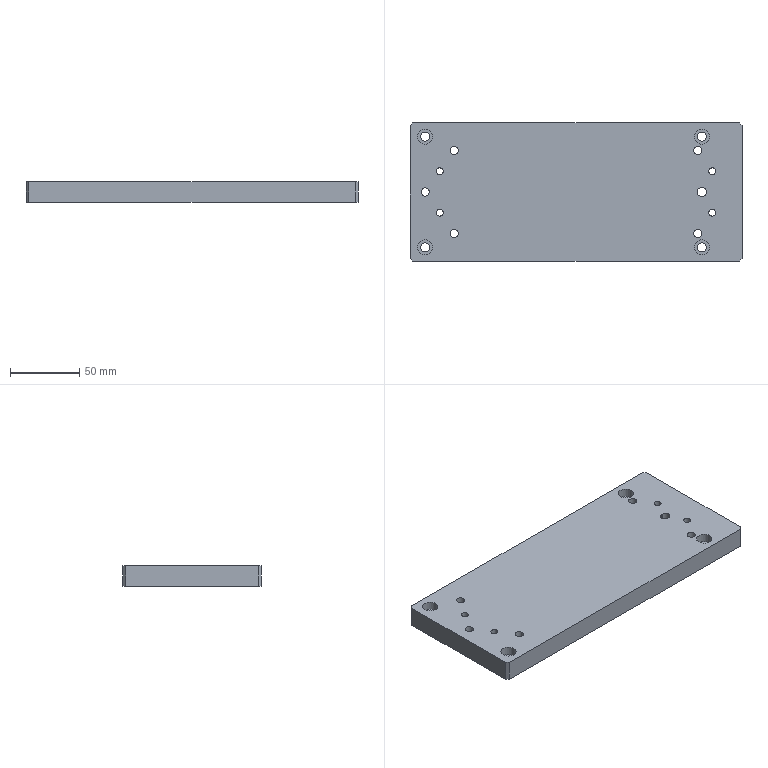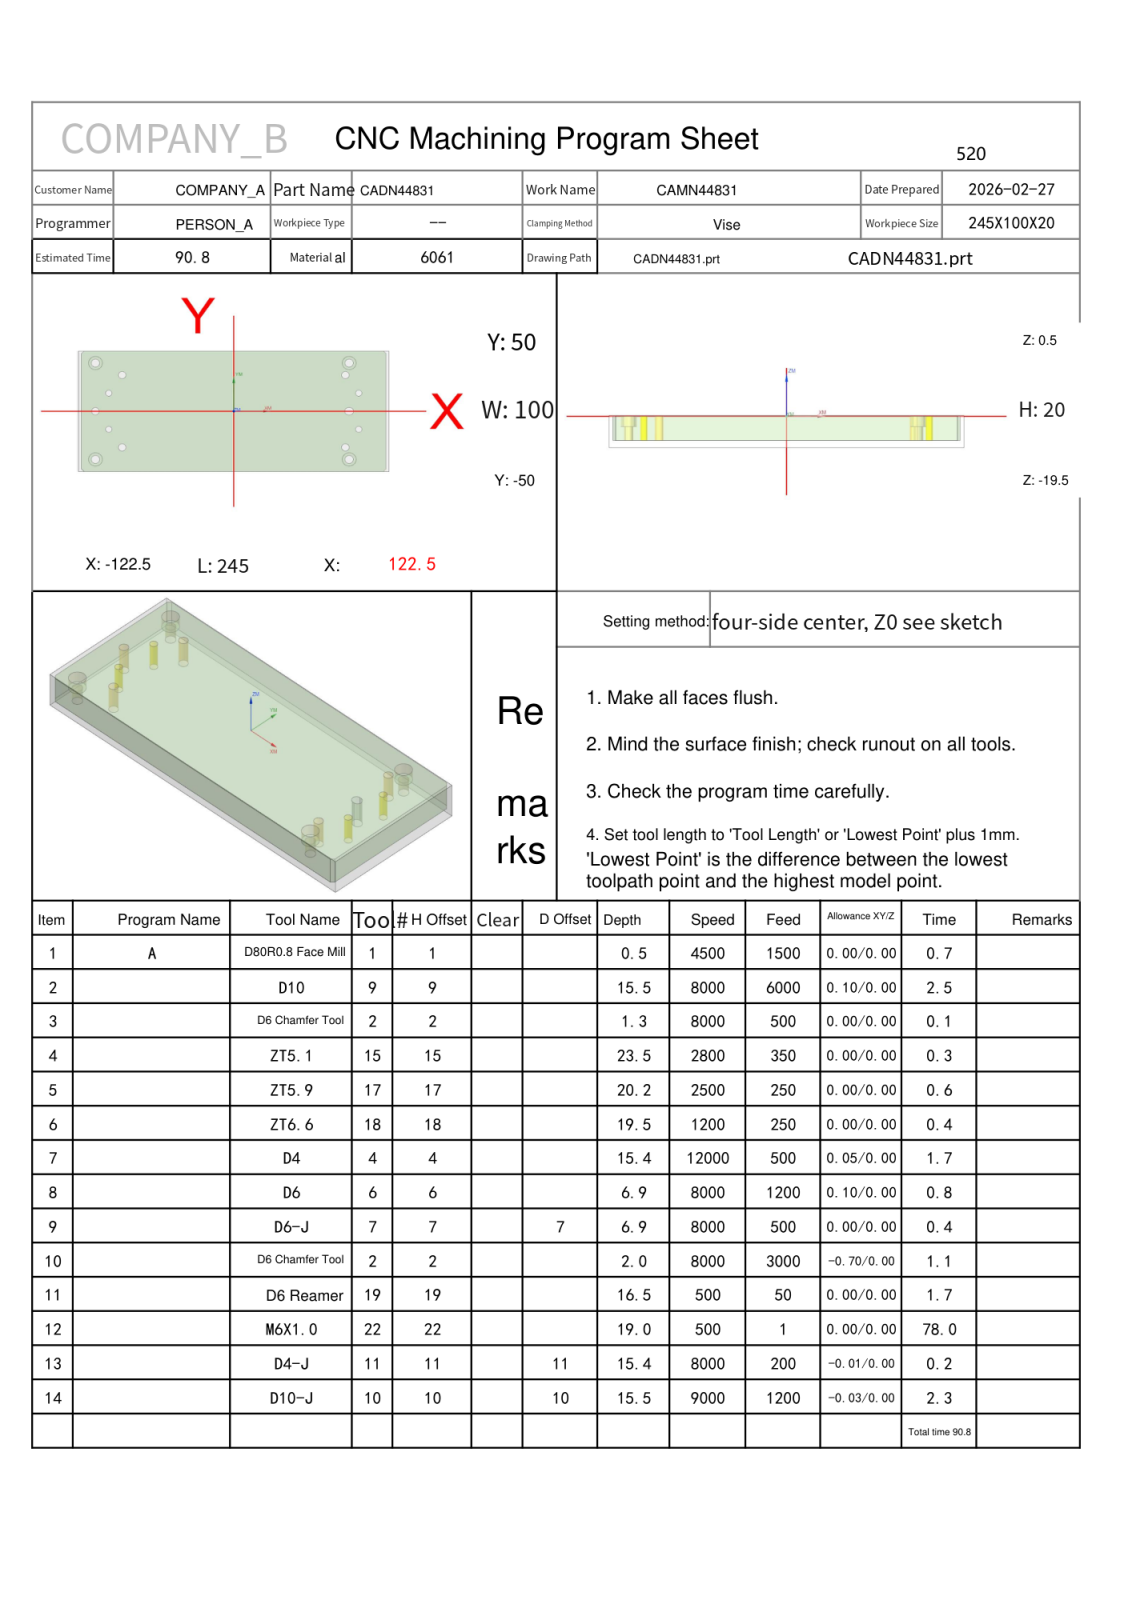NC program | NX | posted by the shop | part box 240 x 100 x 15 mm
Whole program, first 1246 of 1846 lines:
%
O0001
(Machine time: 167.50 MIN)
(===Total Tool:13===)
(T1=D80R0.8-FaceMill D=80.  R=0.8  D-  H01 Z=0.    )
(T9=D10     D=10.  R=0.   D-  H09 Z=-15.  )
(T2=D6_ChamferTool   D=6.   R=0.   D-  H02 Z=-1.5  )
(T15=ZT5.1  D=5.1  DR_a=118 D-  H15 Z=-23.  )
(T17=ZT5.9  D=5.9  DR_a=120 D-  H17 Z=-19.7 )
(T18=ZT6.6  D=6.6  DR_a=118 D-  H18 Z=-18.98)
(T4=D4      D=4.   R=0.   D-  H04 Z=-14.9 )
(T6=D6      D=6.   R=0.   D-  H06 Z=-6.4  )
(T7=D6-J    D=6.   R=0.   D7  H07 Z=-6.4  )
(T19=D6_Reamer   D=6.   DR_a=180 D-  H19 Z=-16.  )
(T22=M6X1.0 D=5.   DR_a=180 D-  H22 Z=-18.5 )
(T11=D4-J   D=4.   R=0.   D11 H11 Z=-14.9 )
(T10=D10-J  D=10.  R=0.   D10 H10 Z=-15.  )
G80 G90 G17 G49 G40
G91 G28 Z0
M01
N1 T01 M06
(D80R0.8-FaceMill  D=80. R=0.8 H=01 ce=0.00 di=0.00)
G00 G90 G54 X-165. Y45. M03 S4500
G43 H01 Z50.
M08
Z2.
G01 Z0.0 F1500.
X-160.
X160.
Y0.0
X-160.
Y-45.
X160.
X165.
Z2.
G00 Z50.
G91 G28 Z0.0
M05
M09
G91 G28 Z0.0
M01
N2 T09 M06
(D10  D=10. R=0. H=09 ce=0.10 di=0.00)
G00 G90 G54 X0.0 Y55.1 M03 S8000
G43 H09 Z50.
M08
Z.5
G01 X118. Z.371 F6000.
G02 X121.606 Y53.606 Z.366 I0.0 J-5.1
G01 X123.606 Y51.606 Z.363
G02 X125.1 Y48. Z.359 I-3.606 J-3.606
G01 Y-48. Z.254
G02 X123.606 Y-51.606 Z.249 I-5.1 J0.0
G01 X121.606 Y-53.606 Z.246
G02 X118. Y-55.1 Z.242 I-3.606 J3.606
G01 X-118. Z-.017
G02 X-121.606 Y-53.606 Z-.021 I0.0 J5.1
G01 X-123.606 Y-51.606 Z-.024
G02 X-125.1 Y-48. Z-.029 I3.606 J3.606
G01 Y48. Z-.134
G02 X-123.606 Y51.606 Z-.138 I5.1 J0.0
G01 X-121.606 Y53.606 Z-.141
G02 X-118. Y55.1 Z-.146 I3.606 J-3.606
G01 X118. Z-.404
G02 X121.606 Y53.606 Z-.409 I0.0 J-5.1
G01 X123.606 Y51.606 Z-.412
G02 X125.1 Y48. Z-.416 I-3.606 J-3.606
G01 Y-48. Z-.521
G02 X123.606 Y-51.606 Z-.526 I-5.1 J0.0
G01 X121.606 Y-53.606 Z-.529
G02 X118. Y-55.1 Z-.533 I-3.606 J3.606
G01 X-118. Z-.792
G02 X-121.606 Y-53.606 Z-.796 I0.0 J5.1
G01 X-123.606 Y-51.606 Z-.799
G02 X-125.1 Y-48. Z-.804 I3.606 J3.606
G01 Y48. Z-.909
G02 X-123.606 Y51.606 Z-.913 I5.1 J0.0
G01 X-121.606 Y53.606 Z-.916
G02 X-118. Y55.1 Z-.921 I3.606 J-3.606
G01 X118. Z-1.179
G02 X121.606 Y53.606 Z-1.184 I0.0 J-5.1
G01 X123.606 Y51.606 Z-1.187
G02 X125.1 Y48. Z-1.191 I-3.606 J-3.606
G01 Y-48. Z-1.296
G02 X123.606 Y-51.606 Z-1.301 I-5.1 J0.0
G01 X121.606 Y-53.606 Z-1.304
G02 X118. Y-55.1 Z-1.308 I-3.606 J3.606
G01 X-118. Z-1.567
G02 X-121.606 Y-53.606 Z-1.571 I0.0 J5.1
G01 X-123.606 Y-51.606 Z-1.574
G02 X-125.1 Y-48. Z-1.579 I3.606 J3.606
G01 Y48. Z-1.684
G02 X-123.606 Y51.606 Z-1.688 I5.1 J0.0
G01 X-121.606 Y53.606 Z-1.691
G02 X-118. Y55.1 Z-1.696 I3.606 J-3.606
G01 X118. Z-1.954
G02 X121.606 Y53.606 Z-1.959 I0.0 J-5.1
G01 X123.606 Y51.606 Z-1.962
G02 X125.1 Y48. Z-1.966 I-3.606 J-3.606
G01 Y-48. Z-2.071
G02 X123.606 Y-51.606 Z-2.076 I-5.1 J0.0
G01 X121.606 Y-53.606 Z-2.079
G02 X118. Y-55.1 Z-2.083 I-3.606 J3.606
G01 X-118. Z-2.342
G02 X-121.606 Y-53.606 Z-2.346 I0.0 J5.1
G01 X-123.606 Y-51.606 Z-2.349
G02 X-125.1 Y-48. Z-2.354 I3.606 J3.606
G01 Y48. Z-2.459
G02 X-123.606 Y51.606 Z-2.463 I5.1 J0.0
G01 X-121.606 Y53.606 Z-2.466
G02 X-118. Y55.1 Z-2.471 I3.606 J-3.606
G01 X118. Z-2.729
G02 X121.606 Y53.606 Z-2.734 I0.0 J-5.1
G01 X123.606 Y51.606 Z-2.737
G02 X125.1 Y48. Z-2.741 I-3.606 J-3.606
G01 Y-48. Z-2.846
G02 X123.606 Y-51.606 Z-2.851 I-5.1 J0.0
G01 X121.606 Y-53.606 Z-2.854
G02 X118. Y-55.1 Z-2.858 I-3.606 J3.606
G01 X-118. Z-3.117
G02 X-121.606 Y-53.606 Z-3.121 I0.0 J5.1
G01 X-123.606 Y-51.606 Z-3.124
G02 X-125.1 Y-48. Z-3.129 I3.606 J3.606
G01 Y48. Z-3.234
G02 X-123.606 Y51.606 Z-3.238 I5.1 J0.0
G01 X-121.606 Y53.606 Z-3.241
G02 X-118. Y55.1 Z-3.246 I3.606 J-3.606
G01 X118. Z-3.504
G02 X121.606 Y53.606 Z-3.509 I0.0 J-5.1
G01 X123.606 Y51.606 Z-3.512
G02 X125.1 Y48. Z-3.516 I-3.606 J-3.606
G01 Y-48. Z-3.621
G02 X123.606 Y-51.606 Z-3.626 I-5.1 J0.0
G01 X121.606 Y-53.606 Z-3.629
G02 X118. Y-55.1 Z-3.633 I-3.606 J3.606
G01 X-118. Z-3.892
G02 X-121.606 Y-53.606 Z-3.896 I0.0 J5.1
G01 X-123.606 Y-51.606 Z-3.899
G02 X-125.1 Y-48. Z-3.904 I3.606 J3.606
G01 Y48. Z-4.009
G02 X-123.606 Y51.606 Z-4.013 I5.1 J0.0
G01 X-121.606 Y53.606 Z-4.016
G02 X-118. Y55.1 Z-4.021 I3.606 J-3.606
G01 X118. Z-4.279
G02 X121.606 Y53.606 Z-4.284 I0.0 J-5.1
G01 X123.606 Y51.606 Z-4.287
G02 X125.1 Y48. Z-4.291 I-3.606 J-3.606
G01 Y-48. Z-4.396
G02 X123.606 Y-51.606 Z-4.401 I-5.1 J0.0
G01 X121.606 Y-53.606 Z-4.404
G02 X118. Y-55.1 Z-4.408 I-3.606 J3.606
G01 X-118. Z-4.667
G02 X-121.606 Y-53.606 Z-4.671 I0.0 J5.1
G01 X-123.606 Y-51.606 Z-4.674
G02 X-125.1 Y-48. Z-4.679 I3.606 J3.606
G01 Y48. Z-4.784
G02 X-123.606 Y51.606 Z-4.788 I5.1 J0.0
G01 X-121.606 Y53.606 Z-4.791
G02 X-118. Y55.1 Z-4.796 I3.606 J-3.606
G01 X118. Z-5.054
G02 X121.606 Y53.606 Z-5.059 I0.0 J-5.1
G01 X123.606 Y51.606 Z-5.062
G02 X125.1 Y48. Z-5.066 I-3.606 J-3.606
G01 Y-48. Z-5.171
G02 X123.606 Y-51.606 Z-5.176 I-5.1 J0.0
G01 X121.606 Y-53.606 Z-5.179
G02 X118. Y-55.1 Z-5.183 I-3.606 J3.606
G01 X-118. Z-5.442
G02 X-121.606 Y-53.606 Z-5.446 I0.0 J5.1
G01 X-123.606 Y-51.606 Z-5.449
G02 X-125.1 Y-48. Z-5.454 I3.606 J3.606
G01 Y48. Z-5.559
G02 X-123.606 Y51.606 Z-5.563 I5.1 J0.0
G01 X-121.606 Y53.606 Z-5.566
G02 X-118. Y55.1 Z-5.571 I3.606 J-3.606
G01 X118. Z-5.829
G02 X121.606 Y53.606 Z-5.834 I0.0 J-5.1
G01 X123.606 Y51.606 Z-5.837
G02 X125.1 Y48. Z-5.841 I-3.606 J-3.606
G01 Y-48. Z-5.946
G02 X123.606 Y-51.606 Z-5.951 I-5.1 J0.0
G01 X121.606 Y-53.606 Z-5.954
G02 X118. Y-55.1 Z-5.958 I-3.606 J3.606
G01 X-118. Z-6.217
G02 X-121.606 Y-53.606 Z-6.221 I0.0 J5.1
G01 X-123.606 Y-51.606 Z-6.224
G02 X-125.1 Y-48. Z-6.229 I3.606 J3.606
G01 Y48. Z-6.334
G02 X-123.606 Y51.606 Z-6.338 I5.1 J0.0
G01 X-121.606 Y53.606 Z-6.341
G02 X-118. Y55.1 Z-6.346 I3.606 J-3.606
G01 X118. Z-6.604
G02 X121.606 Y53.606 Z-6.609 I0.0 J-5.1
G01 X123.606 Y51.606 Z-6.612
G02 X125.1 Y48. Z-6.616 I-3.606 J-3.606
G01 Y-48. Z-6.721
G02 X123.606 Y-51.606 Z-6.726 I-5.1 J0.0
G01 X121.606 Y-53.606 Z-6.729
G02 X118. Y-55.1 Z-6.733 I-3.606 J3.606
G01 X-118. Z-6.992
G02 X-121.606 Y-53.606 Z-6.996 I0.0 J5.1
G01 X-123.606 Y-51.606 Z-6.999
G02 X-125.1 Y-48. Z-7.004 I3.606 J3.606
G01 Y48. Z-7.109
G02 X-123.606 Y51.606 Z-7.113 I5.1 J0.0
G01 X-121.606 Y53.606 Z-7.116
G02 X-118. Y55.1 Z-7.121 I3.606 J-3.606
G01 X118. Z-7.379
G02 X121.606 Y53.606 Z-7.384 I0.0 J-5.1
G01 X123.606 Y51.606 Z-7.387
G02 X125.1 Y48. Z-7.391 I-3.606 J-3.606
G01 Y-48. Z-7.496
G02 X123.606 Y-51.606 Z-7.501 I-5.1 J0.0
G01 X121.606 Y-53.606 Z-7.504
G02 X118. Y-55.1 Z-7.508 I-3.606 J3.606
G01 X-118. Z-7.767
G02 X-121.606 Y-53.606 Z-7.771 I0.0 J5.1
G01 X-123.606 Y-51.606 Z-7.774
G02 X-125.1 Y-48. Z-7.779 I3.606 J3.606
G01 Y48. Z-7.884
G02 X-123.606 Y51.606 Z-7.888 I5.1 J0.0
G01 X-121.606 Y53.606 Z-7.891
G02 X-118. Y55.1 Z-7.896 I3.606 J-3.606
G01 X118. Z-8.154
G02 X121.606 Y53.606 Z-8.159 I0.0 J-5.1
G01 X123.606 Y51.606 Z-8.162
G02 X125.1 Y48. Z-8.166 I-3.606 J-3.606
G01 Y-48. Z-8.271
G02 X123.606 Y-51.606 Z-8.276 I-5.1 J0.0
G01 X121.606 Y-53.606 Z-8.279
G02 X118. Y-55.1 Z-8.283 I-3.606 J3.606
G01 X-118. Z-8.542
G02 X-121.606 Y-53.606 Z-8.546 I0.0 J5.1
G01 X-123.606 Y-51.606 Z-8.549
G02 X-125.1 Y-48. Z-8.554 I3.606 J3.606
G01 Y48. Z-8.659
G02 X-123.606 Y51.606 Z-8.663 I5.1 J0.0
G01 X-121.606 Y53.606 Z-8.666
G02 X-118. Y55.1 Z-8.671 I3.606 J-3.606
G01 X118. Z-8.929
G02 X121.606 Y53.606 Z-8.934 I0.0 J-5.1
G01 X123.606 Y51.606 Z-8.937
G02 X125.1 Y48. Z-8.941 I-3.606 J-3.606
G01 Y-48. Z-9.046
G02 X123.606 Y-51.606 Z-9.051 I-5.1 J0.0
G01 X121.606 Y-53.606 Z-9.054
G02 X118. Y-55.1 Z-9.058 I-3.606 J3.606
G01 X-118. Z-9.317
G02 X-121.606 Y-53.606 Z-9.321 I0.0 J5.1
G01 X-123.606 Y-51.606 Z-9.324
G02 X-125.1 Y-48. Z-9.329 I3.606 J3.606
G01 Y48. Z-9.434
G02 X-123.606 Y51.606 Z-9.438 I5.1 J0.0
G01 X-121.606 Y53.606 Z-9.441
G02 X-118. Y55.1 Z-9.446 I3.606 J-3.606
G01 X118. Z-9.704
G02 X121.606 Y53.606 Z-9.709 I0.0 J-5.1
G01 X123.606 Y51.606 Z-9.712
G02 X125.1 Y48. Z-9.716 I-3.606 J-3.606
G01 Y-48. Z-9.821
G02 X123.606 Y-51.606 Z-9.826 I-5.1 J0.0
G01 X121.606 Y-53.606 Z-9.829
G02 X118. Y-55.1 Z-9.833 I-3.606 J3.606
G01 X-118. Z-10.092
G02 X-121.606 Y-53.606 Z-10.096 I0.0 J5.1
G01 X-123.606 Y-51.606 Z-10.099
G02 X-125.1 Y-48. Z-10.104 I3.606 J3.606
G01 Y48. Z-10.209
G02 X-123.606 Y51.606 Z-10.213 I5.1 J0.0
G01 X-121.606 Y53.606 Z-10.216
G02 X-118. Y55.1 Z-10.221 I3.606 J-3.606
G01 X118. Z-10.479
G02 X121.606 Y53.606 Z-10.484 I0.0 J-5.1
G01 X123.606 Y51.606 Z-10.487
G02 X125.1 Y48. Z-10.491 I-3.606 J-3.606
G01 Y-48. Z-10.596
G02 X123.606 Y-51.606 Z-10.601 I-5.1 J0.0
G01 X121.606 Y-53.606 Z-10.604
G02 X118. Y-55.1 Z-10.608 I-3.606 J3.606
G01 X-118. Z-10.867
G02 X-121.606 Y-53.606 Z-10.871 I0.0 J5.1
G01 X-123.606 Y-51.606 Z-10.874
G02 X-125.1 Y-48. Z-10.879 I3.606 J3.606
G01 Y48. Z-10.984
G02 X-123.606 Y51.606 Z-10.988 I5.1 J0.0
G01 X-121.606 Y53.606 Z-10.991
G02 X-118. Y55.1 Z-10.996 I3.606 J-3.606
G01 X118. Z-11.254
G02 X121.606 Y53.606 Z-11.259 I0.0 J-5.1
G01 X123.606 Y51.606 Z-11.262
G02 X125.1 Y48. Z-11.266 I-3.606 J-3.606
G01 Y-48. Z-11.371
G02 X123.606 Y-51.606 Z-11.376 I-5.1 J0.0
G01 X121.606 Y-53.606 Z-11.379
G02 X118. Y-55.1 Z-11.383 I-3.606 J3.606
G01 X-118. Z-11.642
G02 X-121.606 Y-53.606 Z-11.646 I0.0 J5.1
G01 X-123.606 Y-51.606 Z-11.649
G02 X-125.1 Y-48. Z-11.654 I3.606 J3.606
G01 Y48. Z-11.759
G02 X-123.606 Y51.606 Z-11.763 I5.1 J0.0
G01 X-121.606 Y53.606 Z-11.766
G02 X-118. Y55.1 Z-11.771 I3.606 J-3.606
G01 X118. Z-12.029
G02 X121.606 Y53.606 Z-12.034 I0.0 J-5.1
G01 X123.606 Y51.606 Z-12.037
G02 X125.1 Y48. Z-12.041 I-3.606 J-3.606
G01 Y-48. Z-12.146
G02 X123.606 Y-51.606 Z-12.151 I-5.1 J0.0
G01 X121.606 Y-53.606 Z-12.154
G02 X118. Y-55.1 Z-12.158 I-3.606 J3.606
G01 X-118. Z-12.417
G02 X-121.606 Y-53.606 Z-12.421 I0.0 J5.1
G01 X-123.606 Y-51.606 Z-12.424
G02 X-125.1 Y-48. Z-12.429 I3.606 J3.606
G01 Y48. Z-12.534
G02 X-123.606 Y51.606 Z-12.538 I5.1 J0.0
G01 X-121.606 Y53.606 Z-12.541
G02 X-118. Y55.1 Z-12.546 I3.606 J-3.606
G01 X118. Z-12.804
G02 X121.606 Y53.606 Z-12.809 I0.0 J-5.1
G01 X123.606 Y51.606 Z-12.812
G02 X125.1 Y48. Z-12.816 I-3.606 J-3.606
G01 Y-48. Z-12.921
G02 X123.606 Y-51.606 Z-12.926 I-5.1 J0.0
G01 X121.606 Y-53.606 Z-12.929
G02 X118. Y-55.1 Z-12.933 I-3.606 J3.606
G01 X-118. Z-13.192
G02 X-121.606 Y-53.606 Z-13.196 I0.0 J5.1
G01 X-123.606 Y-51.606 Z-13.199
G02 X-125.1 Y-48. Z-13.204 I3.606 J3.606
G01 Y48. Z-13.309
G02 X-123.606 Y51.606 Z-13.313 I5.1 J0.0
G01 X-121.606 Y53.606 Z-13.316
G02 X-118. Y55.1 Z-13.321 I3.606 J-3.606
G01 X118. Z-13.579
G02 X121.606 Y53.606 Z-13.584 I0.0 J-5.1
G01 X123.606 Y51.606 Z-13.587
G02 X125.1 Y48. Z-13.591 I-3.606 J-3.606
G01 Y-48. Z-13.696
G02 X123.606 Y-51.606 Z-13.701 I-5.1 J0.0
G01 X121.606 Y-53.606 Z-13.704
G02 X118. Y-55.1 Z-13.708 I-3.606 J3.606
G01 X-118. Z-13.967
G02 X-121.606 Y-53.606 Z-13.971 I0.0 J5.1
G01 X-123.606 Y-51.606 Z-13.974
G02 X-125.1 Y-48. Z-13.979 I3.606 J3.606
G01 Y48. Z-14.084
G02 X-123.606 Y51.606 Z-14.088 I5.1 J0.0
G01 X-121.606 Y53.606 Z-14.091
G02 X-118. Y55.1 Z-14.096 I3.606 J-3.606
G01 X118. Z-14.354
G02 X121.606 Y53.606 Z-14.359 I0.0 J-5.1
G01 X123.606 Y51.606 Z-14.362
G02 X125.1 Y48. Z-14.366 I-3.606 J-3.606
G01 Y-48. Z-14.471
G02 X123.606 Y-51.606 Z-14.476 I-5.1 J0.0
G01 X121.606 Y-53.606 Z-14.479
G02 X118. Y-55.1 Z-14.483 I-3.606 J3.606
G01 X-118. Z-14.742
G02 X-121.606 Y-53.606 Z-14.746 I0.0 J5.1
G01 X-123.606 Y-51.606 Z-14.749
G02 X-125.1 Y-48. Z-14.754 I3.606 J3.606
G01 Y48. Z-14.859
G02 X-123.606 Y51.606 Z-14.863 I5.1 J0.0
G01 X-121.606 Y53.606 Z-14.866
G02 X-118. Y55.1 Z-14.871 I3.606 J-3.606
G01 X0.0 Z-15.
X118.
G02 X121.606 Y53.606 I0.0 J-5.1
G01 X123.606 Y51.606
G02 X125.1 Y48. I-3.606 J-3.606
G01 Y-48.
G02 X123.606 Y-51.606 I-5.1 J0.0
G01 X121.606 Y-53.606
G02 X118. Y-55.1 I-3.606 J3.606
G01 X-118.
G02 X-121.606 Y-53.606 I0.0 J5.1
G01 X-123.606 Y-51.606
G02 X-125.1 Y-48. I3.606 J3.606
G01 Y48.
G02 X-123.606 Y51.606 I5.1 J0.0
G01 X-121.606 Y53.606
G02 X-118. Y55.1 I3.606 J-3.606
G01 X0.0
X.5
Z-14.
G00 Z50.
G91 G28 Z0.0
M05
M09
G91 G28 Z0.0
M01
N3 T02 M06
(D6_ChamferTool  D=6. R=0. H=02 ce=0.00 di=0.00)
G00 G90 G54 X91. Y-40. M03 S8000
G43 H02 Z50.
M08
G98 G81 X91. Y-40. Z-.8 R1. F500.
X88. Y-30.
X98.5 Y-15.
Y15.
X88. Y30.
X91. Y40.
X-88. Y30.
X-109. Y40.
X-98.5 Y15.
X-109. Y0.0
X-98.5 Y-15.
X-88. Y-30.
X-109. Y-40.
G80
G00 Z50.
G00 G90 X90.5 Y0.0 M03 S8000
Z50.
G98 G81 X90.5 Y0.0 Z-.8 R1. F500.
G80
G00 Z50.
G91 G28 Z0.0
M05
M09
G91 G28 Z0.0
M01
N4 T15 M06
(ZT5.1 D=5.1 DR_a=118 H=15)
G00 G90 G54 X-98.5 Y15. M03 S2800
G43 H15 Z50.
M08
G98 G83 X-98.5 Y15. Z-23. R1. F350. Q3.
Y-15.
X98.5
Y15.
G80
G00 Z50.
G91 G28 Z0.0
M05
M09
G91 G28 Z0.0
M01
N5 T17 M06
(ZT5.9 D=5.9 DR_a=120 H=17)
G00 G90 G54 X-88. Y-30. M03 S2500
G43 H17 Z50.
M08
G98 G83 X-88. Y-30. Z-19.703 R1. F250. Q2.
X-109. Y0.0
X-88. Y30.
X88.
Y-30.
G80
G00 Z50.
G00 G90 X90.5 Y0.0 M03 S2500
Z50.
G98 G83 X90.5 Y0.0 Z-19.703 R1. F250. Q2.
G80
G00 Z50.
G91 G28 Z0.0
M05
M09
G91 G28 Z0.0
M01
N6 T18 M06
(ZT6.6 D=6.6 DR_a=118 H=18)
G00 G90 G54 X91. Y40. M03 S1200
G43 H18 Z50.
M08
G98 G83 X91. Y40. Z-18.983 R1. F250. Q2.
Y-40.
X-109.
Y40.
G80
G00 Z50.
G91 G28 Z0.0
M05
M09
G91 G28 Z0.0
M01
N7 T04 M06
(D4  D=4. R=0. H=04 ce=0.05 di=0.00)
G00 G90 G54 X91. Y-.95 M03 S12000
G43 H04 Z50.
M08
Z.5
G01 X91.5 Z.491 F500.
G03 X92.45 Y0.0 Z.463 I0.0 J.95
X91.5 Y.95 Z.435 I-.95 J0.0
G01 X90.5 Z.416
G03 X89.55 Y0.0 Z.388 I0.0 J-.95
X90.5 Y-.95 Z.36 I.95 J0.0
G01 X91.5 Z.341
G03 X92.45 Y0.0 Z.313 I0.0 J.95
X91.5 Y.95 Z.285 I-.95 J0.0
G01 X90.5 Z.266
G03 X89.55 Y0.0 Z.238 I0.0 J-.95
X90.5 Y-.95 Z.21 I.95 J0.0
G01 X91.5 Z.192
G03 X92.45 Y0.0 Z.164 I0.0 J.95
X91.5 Y.95 Z.136 I-.95 J0.0
G01 X90.5 Z.117
G03 X89.55 Y0.0 Z.089 I0.0 J-.95
X90.5 Y-.95 Z.061 I.95 J0.0
G01 X91.5 Z.042
G03 X92.45 Y0.0 Z.014 I0.0 J.95
X91.5 Y.95 Z-.014 I-.95 J0.0
G01 X90.5 Z-.033
G03 X89.55 Y0.0 Z-.061 I0.0 J-.95
X90.5 Y-.95 Z-.089 I.95 J0.0
G01 X91.5 Z-.107
G03 X92.45 Y0.0 Z-.135 I0.0 J.95
X91.5 Y.95 Z-.163 I-.95 J0.0
G01 X90.5 Z-.182
G03 X89.55 Y0.0 Z-.21 I0.0 J-.95
X90.5 Y-.95 Z-.238 I.95 J0.0
G01 X91.5 Z-.257
G03 X92.45 Y0.0 Z-.285 I0.0 J.95
X91.5 Y.95 Z-.313 I-.95 J0.0
G01 X90.5 Z-.332
G03 X89.55 Y0.0 Z-.36 I0.0 J-.95
X90.5 Y-.95 Z-.388 I.95 J0.0
G01 X91.5 Z-.406
G03 X92.45 Y0.0 Z-.434 I0.0 J.95
X91.5 Y.95 Z-.462 I-.95 J0.0
G01 X90.5 Z-.481
G03 X89.55 Y0.0 Z-.509 I0.0 J-.95
X90.5 Y-.95 Z-.537 I.95 J0.0
G01 X91.5 Z-.556
G03 X92.45 Y0.0 Z-.584 I0.0 J.95
X91.5 Y.95 Z-.612 I-.95 J0.0
G01 X90.5 Z-.631
G03 X89.55 Y0.0 Z-.659 I0.0 J-.95
X90.5 Y-.95 Z-.687 I.95 J0.0
G01 X91.5 Z-.705
G03 X92.45 Y0.0 Z-.733 I0.0 J.95
X91.5 Y.95 Z-.761 I-.95 J0.0
G01 X90.5 Z-.78
G03 X89.55 Y0.0 Z-.808 I0.0 J-.95
X90.5 Y-.95 Z-.836 I.95 J0.0
G01 X91.5 Z-.855
G03 X92.45 Y0.0 Z-.883 I0.0 J.95
X91.5 Y.95 Z-.911 I-.95 J0.0
G01 X90.5 Z-.93
G03 X89.55 Y0.0 Z-.958 I0.0 J-.95
X90.5 Y-.95 Z-.986 I.95 J0.0
G01 X91.5 Z-1.005
G03 X92.45 Y0.0 Z-1.033 I0.0 J.95
X91.5 Y.95 Z-1.061 I-.95 J0.0
G01 X90.5 Z-1.079
G03 X89.55 Y0.0 Z-1.107 I0.0 J-.95
X90.5 Y-.95 Z-1.135 I.95 J0.0
G01 X91.5 Z-1.154
G03 X92.45 Y0.0 Z-1.182 I0.0 J.95
X91.5 Y.95 Z-1.21 I-.95 J0.0
G01 X90.5 Z-1.229
G03 X89.55 Y0.0 Z-1.257 I0.0 J-.95
X90.5 Y-.95 Z-1.285 I.95 J0.0
G01 X91.5 Z-1.304
G03 X92.45 Y0.0 Z-1.332 I0.0 J.95
X91.5 Y.95 Z-1.36 I-.95 J0.0
G01 X90.5 Z-1.378
G03 X89.55 Y0.0 Z-1.406 I0.0 J-.95
X90.5 Y-.95 Z-1.434 I.95 J0.0
G01 X91.5 Z-1.453
G03 X92.45 Y0.0 Z-1.481 I0.0 J.95
X91.5 Y.95 Z-1.509 I-.95 J0.0
G01 X90.5 Z-1.528
G03 X89.55 Y0.0 Z-1.556 I0.0 J-.95
X90.5 Y-.95 Z-1.584 I.95 J0.0
G01 X91.5 Z-1.603
G03 X92.45 Y0.0 Z-1.631 I0.0 J.95
X91.5 Y.95 Z-1.659 I-.95 J0.0
G01 X90.5 Z-1.677
G03 X89.55 Y0.0 Z-1.705 I0.0 J-.95
X90.5 Y-.95 Z-1.733 I.95 J0.0
G01 X91.5 Z-1.752
G03 X92.45 Y0.0 Z-1.78 I0.0 J.95
X91.5 Y.95 Z-1.808 I-.95 J0.0
G01 X90.5 Z-1.827
G03 X89.55 Y0.0 Z-1.855 I0.0 J-.95
X90.5 Y-.95 Z-1.883 I.95 J0.0
G01 X91.5 Z-1.902
G03 X92.45 Y0.0 Z-1.93 I0.0 J.95
X91.5 Y.95 Z-1.958 I-.95 J0.0
G01 X90.5 Z-1.976
G03 X89.55 Y0.0 Z-2.004 I0.0 J-.95
X90.5 Y-.95 Z-2.032 I.95 J0.0
G01 X91.5 Z-2.051
G03 X92.45 Y0.0 Z-2.079 I0.0 J.95
X91.5 Y.95 Z-2.107 I-.95 J0.0
G01 X90.5 Z-2.126
G03 X89.55 Y0.0 Z-2.154 I0.0 J-.95
X90.5 Y-.95 Z-2.182 I.95 J0.0
G01 X91.5 Z-2.201
G03 X92.45 Y0.0 Z-2.229 I0.0 J.95
X91.5 Y.95 Z-2.257 I-.95 J0.0
G01 X90.5 Z-2.275
G03 X89.55 Y0.0 Z-2.303 I0.0 J-.95
X90.5 Y-.95 Z-2.331 I.95 J0.0
G01 X91.5 Z-2.35
G03 X92.45 Y0.0 Z-2.378 I0.0 J.95
X91.5 Y.95 Z-2.406 I-.95 J0.0
G01 X90.5 Z-2.425
G03 X89.55 Y0.0 Z-2.453 I0.0 J-.95
X90.5 Y-.95 Z-2.481 I.95 J0.0
G01 X91.5 Z-2.5
G03 X92.45 Y0.0 Z-2.528 I0.0 J.95
X91.5 Y.95 Z-2.556 I-.95 J0.0
G01 X90.5 Z-2.574
G03 X89.55 Y0.0 Z-2.602 I0.0 J-.95
X90.5 Y-.95 Z-2.63 I.95 J0.0
G01 X91.5 Z-2.649
G03 X92.45 Y0.0 Z-2.677 I0.0 J.95
X91.5 Y.95 Z-2.705 I-.95 J0.0
G01 X90.5 Z-2.724
G03 X89.55 Y0.0 Z-2.752 I0.0 J-.95
X90.5 Y-.95 Z-2.78 I.95 J0.0
G01 X91.5 Z-2.799
G03 X92.45 Y0.0 Z-2.827 I0.0 J.95
X91.5 Y.95 Z-2.855 I-.95 J0.0
G01 X90.5 Z-2.873
G03 X89.55 Y0.0 Z-2.901 I0.0 J-.95
X90.5 Y-.95 Z-2.929 I.95 J0.0
G01 X91.5 Z-2.948
G03 X92.45 Y0.0 Z-2.976 I0.0 J.95
X91.5 Y.95 Z-3.004 I-.95 J0.0
G01 X90.5 Z-3.023
G03 X89.55 Y0.0 Z-3.051 I0.0 J-.95
X90.5 Y-.95 Z-3.079 I.95 J0.0
G01 X91.5 Z-3.098
G03 X92.45 Y0.0 Z-3.126 I0.0 J.95
X91.5 Y.95 Z-3.154 I-.95 J0.0
G01 X90.5 Z-3.172
G03 X89.55 Y0.0 Z-3.2 I0.0 J-.95
X90.5 Y-.95 Z-3.228 I.95 J0.0
G01 X91.5 Z-3.247
G03 X92.45 Y0.0 Z-3.275 I0.0 J.95
X91.5 Y.95 Z-3.303 I-.95 J0.0
G01 X90.5 Z-3.322
G03 X89.55 Y0.0 Z-3.35 I0.0 J-.95
X90.5 Y-.95 Z-3.378 I.95 J0.0
G01 X91.5 Z-3.397
G03 X92.45 Y0.0 Z-3.425 I0.0 J.95
X91.5 Y.95 Z-3.453 I-.95 J0.0
G01 X90.5 Z-3.472
G03 X89.55 Y0.0 Z-3.5 I0.0 J-.95
X90.5 Y-.95 Z-3.528 I.95 J0.0
G01 X91.5 Z-3.546
G03 X92.45 Y0.0 Z-3.574 I0.0 J.95
X91.5 Y.95 Z-3.602 I-.95 J0.0
G01 X90.5 Z-3.621
G03 X89.55 Y0.0 Z-3.649 I0.0 J-.95
X90.5 Y-.95 Z-3.677 I.95 J0.0
G01 X91.5 Z-3.696
G03 X92.45 Y0.0 Z-3.724 I0.0 J.95
X91.5 Y.95 Z-3.752 I-.95 J0.0
G01 X90.5 Z-3.771
G03 X89.55 Y0.0 Z-3.799 I0.0 J-.95
X90.5 Y-.95 Z-3.827 I.95 J0.0
G01 X91.5 Z-3.845
G03 X92.45 Y0.0 Z-3.873 I0.0 J.95
X91.5 Y.95 Z-3.901 I-.95 J0.0
G01 X90.5 Z-3.92
G03 X89.55 Y0.0 Z-3.948 I0.0 J-.95
X90.5 Y-.95 Z-3.976 I.95 J0.0
G01 X91.5 Z-3.995
G03 X92.45 Y0.0 Z-4.023 I0.0 J.95
X91.5 Y.95 Z-4.051 I-.95 J0.0
G01 X90.5 Z-4.07
G03 X89.55 Y0.0 Z-4.098 I0.0 J-.95
X90.5 Y-.95 Z-4.126 I.95 J0.0
G01 X91.5 Z-4.144
G03 X92.45 Y0.0 Z-4.172 I0.0 J.95
X91.5 Y.95 Z-4.2 I-.95 J0.0
G01 X90.5 Z-4.219
G03 X89.55 Y0.0 Z-4.247 I0.0 J-.95
X90.5 Y-.95 Z-4.275 I.95 J0.0
G01 X91.5 Z-4.294
G03 X92.45 Y0.0 Z-4.322 I0.0 J.95
X91.5 Y.95 Z-4.35 I-.95 J0.0
G01 X90.5 Z-4.369
G03 X89.55 Y0.0 Z-4.397 I0.0 J-.95
X90.5 Y-.95 Z-4.425 I.95 J0.0
G01 X91.5 Z-4.443
G03 X92.45 Y0.0 Z-4.471 I0.0 J.95
X91.5 Y.95 Z-4.499 I-.95 J0.0
G01 X90.5 Z-4.518
G03 X89.55 Y0.0 Z-4.546 I0.0 J-.95
X90.5 Y-.95 Z-4.574 I.95 J0.0
G01 X91.5 Z-4.593
G03 X92.45 Y0.0 Z-4.621 I0.0 J.95
X91.5 Y.95 Z-4.649 I-.95 J0.0
G01 X90.5 Z-4.668
G03 X89.55 Y0.0 Z-4.696 I0.0 J-.95
X90.5 Y-.95 Z-4.724 I.95 J0.0
G01 X91.5 Z-4.742
G03 X92.45 Y0.0 Z-4.77 I0.0 J.95
X91.5 Y.95 Z-4.798 I-.95 J0.0
G01 X90.5 Z-4.817
G03 X89.55 Y0.0 Z-4.845 I0.0 J-.95
X90.5 Y-.95 Z-4.873 I.95 J0.0
G01 X91.5 Z-4.892
G03 X92.45 Y0.0 Z-4.92 I0.0 J.95
X91.5 Y.95 Z-4.948 I-.95 J0.0
G01 X90.5 Z-4.967
G03 X89.55 Y0.0 Z-4.995 I0.0 J-.95
X90.5 Y-.95 Z-5.023 I.95 J0.0
G01 X91.5 Z-5.041
G03 X92.45 Y0.0 Z-5.069 I0.0 J.95
X91.5 Y.95 Z-5.097 I-.95 J0.0
G01 X90.5 Z-5.116
G03 X89.55 Y0.0 Z-5.144 I0.0 J-.95
X90.5 Y-.95 Z-5.172 I.95 J0.0
G01 X91.5 Z-5.191
G03 X92.45 Y0.0 Z-5.219 I0.0 J.95
X91.5 Y.95 Z-5.247 I-.95 J0.0
G01 X90.5 Z-5.266
G03 X89.55 Y0.0 Z-5.294 I0.0 J-.95
X90.5 Y-.95 Z-5.322 I.95 J0.0
G01 X91.5 Z-5.34
G03 X92.45 Y0.0 Z-5.368 I0.0 J.95
X91.5 Y.95 Z-5.396 I-.95 J0.0
G01 X90.5 Z-5.415
G03 X89.55 Y0.0 Z-5.443 I0.0 J-.95
X90.5 Y-.95 Z-5.471 I.95 J0.0
G01 X91.5 Z-5.49
G03 X92.45 Y0.0 Z-5.518 I0.0 J.95
X91.5 Y.95 Z-5.546 I-.95 J0.0
G01 X90.5 Z-5.565
G03 X89.55 Y0.0 Z-5.593 I0.0 J-.95
X90.5 Y-.95 Z-5.621 I.95 J0.0
G01 X91.5 Z-5.639
G03 X92.45 Y0.0 Z-5.667 I0.0 J.95
X91.5 Y.95 Z-5.695 I-.95 J0.0
G01 X90.5 Z-5.714
G03 X89.55 Y0.0 Z-5.742 I0.0 J-.95
X90.5 Y-.95 Z-5.77 I.95 J0.0
G01 X91.5 Z-5.789
G03 X92.45 Y0.0 Z-5.817 I0.0 J.95
X91.5 Y.95 Z-5.845 I-.95 J0.0
G01 X90.5 Z-5.864
G03 X89.55 Y0.0 Z-5.892 I0.0 J-.95
X90.5 Y-.95 Z-5.92 I.95 J0.0
G01 X91.5 Z-5.939
G03 X92.45 Y0.0 Z-5.967 I0.0 J.95
X91.5 Y.95 Z-5.995 I-.95 J0.0
G01 X90.5 Z-6.013
G03 X89.55 Y0.0 Z-6.041 I0.0 J-.95
X90.5 Y-.95 Z-6.069 I.95 J0.0
G01 X91.5 Z-6.088
G03 X92.45 Y0.0 Z-6.116 I0.0 J.95
X91.5 Y.95 Z-6.144 I-.95 J0.0
G01 X90.5 Z-6.163
G03 X89.55 Y0.0 Z-6.191 I0.0 J-.95
X90.5 Y-.95 Z-6.219 I.95 J0.0
G01 X91.5 Z-6.238
G03 X92.45 Y0.0 Z-6.266 I0.0 J.95
X91.5 Y.95 Z-6.294 I-.95 J0.0
G01 X90.5 Z-6.312
G03 X89.55 Y0.0 Z-6.34 I0.0 J-.95
X90.5 Y-.95 Z-6.368 I.95 J0.0
G01 X91.5 Z-6.387
G03 X92.45 Y0.0 Z-6.415 I0.0 J.95
X91.5 Y.95 Z-6.443 I-.95 J0.0
G01 X90.5 Z-6.462
G03 X89.55 Y0.0 Z-6.49 I0.0 J-.95
X90.5 Y-.95 Z-6.518 I.95 J0.0
G01 X91.5 Z-6.537
G03 X92.45 Y0.0 Z-6.565 I0.0 J.95
X91.5 Y.95 Z-6.593 I-.95 J0.0
G01 X90.5 Z-6.611
G03 X89.55 Y0.0 Z-6.639 I0.0 J-.95
X90.5 Y-.95 Z-6.667 I.95 J0.0
G01 X91.5 Z-6.686
G03 X92.45 Y0.0 Z-6.714 I0.0 J.95
X91.5 Y.95 Z-6.742 I-.95 J0.0
G01 X90.5 Z-6.761
G03 X89.55 Y0.0 Z-6.789 I0.0 J-.95
X90.5 Y-.95 Z-6.817 I.95 J0.0
G01 X91.5 Z-6.836
G03 X92.45 Y0.0 Z-6.864 I0.0 J.95
X91.5 Y.95 Z-6.892 I-.95 J0.0
G01 X90.5 Z-6.91
G03 X89.55 Y0.0 Z-6.938 I0.0 J-.95
X90.5 Y-.95 Z-6.966 I.95 J0.0
G01 X91.5 Z-6.985
G03 X92.45 Y0.0 Z-7.013 I0.0 J.95
X91.5 Y.95 Z-7.041 I-.95 J0.0
G01 X90.5 Z-7.06
G03 X89.55 Y0.0 Z-7.088 I0.0 J-.95
X90.5 Y-.95 Z-7.116 I.95 J0.0
G01 X91.5 Z-7.135
G03 X92.45 Y0.0 Z-7.163 I0.0 J.95
X91.5 Y.95 Z-7.191 I-.95 J0.0
G01 X90.5 Z-7.209
G03 X89.55 Y0.0 Z-7.237 I0.0 J-.95
X90.5 Y-.95 Z-7.265 I.95 J0.0
G01 X91.5 Z-7.284
G03 X92.45 Y0.0 Z-7.312 I0.0 J.95
X91.5 Y.95 Z-7.34 I-.95 J0.0
G01 X90.5 Z-7.359
G03 X89.55 Y0.0 Z-7.387 I0.0 J-.95
X90.5 Y-.95 Z-7.415 I.95 J0.0
G01 X91.5 Z-7.434
G03 X92.45 Y0.0 Z-7.462 I0.0 J.95
X91.5 Y.95 Z-7.49 I-.95 J0.0
G01 X90.5 Z-7.508
G03 X89.55 Y0.0 Z-7.536 I0.0 J-.95
X90.5 Y-.95 Z-7.564 I.95 J0.0
G01 X91.5 Z-7.583
G03 X92.45 Y0.0 Z-7.611 I0.0 J.95
X91.5 Y.95 Z-7.639 I-.95 J0.0
G01 X90.5 Z-7.658
G03 X89.55 Y0.0 Z-7.686 I0.0 J-.95
X90.5 Y-.95 Z-7.714 I.95 J0.0
G01 X91.5 Z-7.733
G03 X92.45 Y0.0 Z-7.761 I0.0 J.95
X91.5 Y.95 Z-7.789 I-.95 J0.0
G01 X90.5 Z-7.807
G03 X89.55 Y0.0 Z-7.835 I0.0 J-.95
X90.5 Y-.95 Z-7.863 I.95 J0.0
G01 X91.5 Z-7.882
G03 X92.45 Y0.0 Z-7.91 I0.0 J.95
X91.5 Y.95 Z-7.938 I-.95 J0.0
G01 X90.5 Z-7.957
G03 X89.55 Y0.0 Z-7.985 I0.0 J-.95
X90.5 Y-.95 Z-8.013 I.95 J0.0
G01 X91.5 Z-8.032
G03 X92.45 Y0.0 Z-8.06 I0.0 J.95
X91.5 Y.95 Z-8.088 I-.95 J0.0
G01 X90.5 Z-8.106
G03 X89.55 Y0.0 Z-8.134 I0.0 J-.95
X90.5 Y-.95 Z-8.162 I.95 J0.0
G01 X91.5 Z-8.181
G03 X92.45 Y0.0 Z-8.209 I0.0 J.95
X91.5 Y.95 Z-8.237 I-.95 J0.0
G01 X90.5 Z-8.256
G03 X89.55 Y0.0 Z-8.284 I0.0 J-.95
X90.5 Y-.95 Z-8.312 I.95 J0.0
G01 X91.5 Z-8.331
G03 X92.45 Y0.0 Z-8.359 I0.0 J.95
X91.5 Y.95 Z-8.387 I-.95 J0.0
G01 X90.5 Z-8.405
G03 X89.55 Y0.0 Z-8.433 I0.0 J-.95
X90.5 Y-.95 Z-8.461 I.95 J0.0
G01 X91.5 Z-8.48
G03 X92.45 Y0.0 Z-8.508 I0.0 J.95
X91.5 Y.95 Z-8.536 I-.95 J0.0
G01 X90.5 Z-8.555
G03 X89.55 Y0.0 Z-8.583 I0.0 J-.95
X90.5 Y-.95 Z-8.611 I.95 J0.0
G01 X91.5 Z-8.63
G03 X92.45 Y0.0 Z-8.658 I0.0 J.95
X91.5 Y.95 Z-8.686 I-.95 J0.0
G01 X90.5 Z-8.705
G03 X89.55 Y0.0 Z-8.733 I0.0 J-.95
X90.5 Y-.95 Z-8.761 I.95 J0.0
G01 X91.5 Z-8.779
G03 X92.45 Y0.0 Z-8.807 I0.0 J.95
X91.5 Y.95 Z-8.835 I-.95 J0.0
G01 X90.5 Z-8.854
G03 X89.55 Y0.0 Z-8.882 I0.0 J-.95
X90.5 Y-.95 Z-8.91 I.95 J0.0
G01 X91.5 Z-8.929
G03 X92.45 Y0.0 Z-8.957 I0.0 J.95
X91.5 Y.95 Z-8.985 I-.95 J0.0
G01 X90.5 Z-9.004
G03 X89.55 Y0.0 Z-9.032 I0.0 J-.95
X90.5 Y-.95 Z-9.06 I.95 J0.0
G01 X91.5 Z-9.078
G03 X92.45 Y0.0 Z-9.106 I0.0 J.95
X91.5 Y.95 Z-9.134 I-.95 J0.0
G01 X90.5 Z-9.153
G03 X89.55 Y0.0 Z-9.181 I0.0 J-.95
X90.5 Y-.95 Z-9.209 I.95 J0.0
G01 X91.5 Z-9.228
G03 X92.45 Y0.0 Z-9.256 I0.0 J.95
X91.5 Y.95 Z-9.284 I-.95 J0.0
G01 X90.5 Z-9.303
G03 X89.55 Y0.0 Z-9.331 I0.0 J-.95
X90.5 Y-.95 Z-9.359 I.95 J0.0
G01 X91.5 Z-9.377
G03 X92.45 Y0.0 Z-9.405 I0.0 J.95
X91.5 Y.95 Z-9.433 I-.95 J0.0
G01 X90.5 Z-9.452
G03 X89.55 Y0.0 Z-9.48 I0.0 J-.95
X90.5 Y-.95 Z-9.508 I.95 J0.0
G01 X91.5 Z-9.527
G03 X92.45 Y0.0 Z-9.555 I0.0 J.95
X91.5 Y.95 Z-9.583 I-.95 J0.0
G01 X90.5 Z-9.602
G03 X89.55 Y0.0 Z-9.63 I0.0 J-.95
X90.5 Y-.95 Z-9.658 I.95 J0.0
G01 X91.5 Z-9.676
G03 X92.45 Y0.0 Z-9.704 I0.0 J.95
X91.5 Y.95 Z-9.732 I-.95 J0.0
G01 X90.5 Z-9.751
G03 X89.55 Y0.0 Z-9.779 I0.0 J-.95
X90.5 Y-.95 Z-9.807 I.95 J0.0
G01 X91.5 Z-9.826
G03 X92.45 Y0.0 Z-9.854 I0.0 J.95
X91.5 Y.95 Z-9.882 I-.95 J0.0
G01 X90.5 Z-9.901
G03 X89.55 Y0.0 Z-9.929 I0.0 J-.95
X90.5 Y-.95 Z-9.957 I.95 J0.0
G01 X91.5 Z-9.975
G03 X92.45 Y0.0 Z-10.003 I0.0 J.95
X91.5 Y.95 Z-10.031 I-.95 J0.0
G01 X90.5 Z-10.05
G03 X89.55 Y0.0 Z-10.078 I0.0 J-.95
X90.5 Y-.95 Z-10.106 I.95 J0.0
G01 X91.5 Z-10.125
G03 X92.45 Y0.0 Z-10.153 I0.0 J.95
X91.5 Y.95 Z-10.181 I-.95 J0.0
G01 X90.5 Z-10.2
G03 X89.55 Y0.0 Z-10.228 I0.0 J-.95
X90.5 Y-.95 Z-10.256 I.95 J0.0
G01 X91.5 Z-10.274
G03 X92.45 Y0.0 Z-10.302 I0.0 J.95
X91.5 Y.95 Z-10.33 I-.95 J0.0
G01 X90.5 Z-10.349
G03 X89.55 Y0.0 Z-10.377 I0.0 J-.95
X90.5 Y-.95 Z-10.405 I.95 J0.0
G01 X91.5 Z-10.424
G03 X92.45 Y0.0 Z-10.452 I0.0 J.95
X91.5 Y.95 Z-10.48 I-.95 J0.0
G01 X90.5 Z-10.499
G03 X89.55 Y0.0 Z-10.527 I0.0 J-.95
X90.5 Y-.95 Z-10.555 I.95 J0.0
G01 X91.5 Z-10.573
G03 X92.45 Y0.0 Z-10.601 I0.0 J.95
X91.5 Y.95 Z-10.629 I-.95 J0.0
G01 X90.5 Z-10.648
G03 X89.55 Y0.0 Z-10.676 I0.0 J-.95
X90.5 Y-.95 Z-10.704 I.95 J0.0
G01 X91.5 Z-10.723
G03 X92.45 Y0.0 Z-10.751 I0.0 J.95
X91.5 Y.95 Z-10.779 I-.95 J0.0
G01 X90.5 Z-10.798
G03 X89.55 Y0.0 Z-10.826 I0.0 J-.95
X90.5 Y-.95 Z-10.854 I.95 J0.0
G01 X91.5 Z-10.872
G03 X92.45 Y0.0 Z-10.9 I0.0 J.95
X91.5 Y.95 Z-10.928 I-.95 J0.0
G01 X90.5 Z-10.947
G03 X89.55 Y0.0 Z-10.975 I0.0 J-.95
X90.5 Y-.95 Z-11.003 I.95 J0.0
G01 X91.5 Z-11.022
G03 X92.45 Y0.0 Z-11.05 I0.0 J.95
X91.5 Y.95 Z-11.078 I-.95 J0.0
G01 X90.5 Z-11.097
G03 X89.55 Y0.0 Z-11.125 I0.0 J-.95
X90.5 Y-.95 Z-11.153 I.95 J0.0
G01 X91.5 Z-11.172
G03 X92.45 Y0.0 Z-11.2 I0.0 J.95
X91.5 Y.95 Z-11.228 I-.95 J0.0
G01 X90.5 Z-11.246
G03 X89.55 Y0.0 Z-11.274 I0.0 J-.95
X90.5 Y-.95 Z-11.302 I.95 J0.0
G01 X91.5 Z-11.321
G03 X92.45 Y0.0 Z-11.349 I0.0 J.95
X91.5 Y.95 Z-11.377 I-.95 J0.0
G01 X90.5 Z-11.396
G03 X89.55 Y0.0 Z-11.424 I0.0 J-.95
X90.5 Y-.95 Z-11.452 I.95 J0.0
G01 X91.5 Z-11.471
G03 X92.45 Y0.0 Z-11.499 I0.0 J.95
X91.5 Y.95 Z-11.527 I-.95 J0.0
G01 X90.5 Z-11.545
G03 X89.55 Y0.0 Z-11.573 I0.0 J-.95
X90.5 Y-.95 Z-11.601 I.95 J0.0
G01 X91.5 Z-11.62
G03 X92.45 Y0.0 Z-11.648 I0.0 J.95
X91.5 Y.95 Z-11.676 I-.95 J0.0
G01 X90.5 Z-11.695
G03 X89.55 Y0.0 Z-11.723 I0.0 J-.95
X90.5 Y-.95 Z-11.751 I.95 J0.0
G01 X91.5 Z-11.77
G03 X92.45 Y0.0 Z-11.798 I0.0 J.95
X91.5 Y.95 Z-11.826 I-.95 J0.0
G01 X90.5 Z-11.844
G03 X89.55 Y0.0 Z-11.872 I0.0 J-.95
X90.5 Y-.95 Z-11.9 I.95 J0.0
G01 X91.5 Z-11.919
G03 X92.45 Y0.0 Z-11.947 I0.0 J.95
X91.5 Y.95 Z-11.975 I-.95 J0.0
G01 X90.5 Z-11.994
G03 X89.55 Y0.0 Z-12.022 I0.0 J-.95
X90.5 Y-.95 Z-12.05 I.95 J0.0
G01 X91.5 Z-12.069
G03 X92.45 Y0.0 Z-12.097 I0.0 J.95
X91.5 Y.95 Z-12.125 I-.95 J0.0
G01 X90.5 Z-12.143
G03 X89.55 Y0.0 Z-12.171 I0.0 J-.95
X90.5 Y-.95 Z-12.199 I.95 J0.0
G01 X91.5 Z-12.218
G03 X92.45 Y0.0 Z-12.246 I0.0 J.95
X91.5 Y.95 Z-12.274 I-.95 J0.0
G01 X90.5 Z-12.293
G03 X89.55 Y0.0 Z-12.321 I0.0 J-.95
X90.5 Y-.95 Z-12.349 I.95 J0.0
G01 X91.5 Z-12.368
G03 X92.45 Y0.0 Z-12.396 I0.0 J.95
X91.5 Y.95 Z-12.424 I-.95 J0.0
G01 X90.5 Z-12.442
G03 X89.55 Y0.0 Z-12.47 I0.0 J-.95
X90.5 Y-.95 Z-12.498 I.95 J0.0
G01 X91.5 Z-12.517
G03 X92.45 Y0.0 Z-12.545 I0.0 J.95
X91.5 Y.95 Z-12.573 I-.95 J0.0
G01 X90.5 Z-12.592
G03 X89.55 Y0.0 Z-12.62 I0.0 J-.95
X90.5 Y-.95 Z-12.648 I.95 J0.0
G01 X91.5 Z-12.667
G03 X92.45 Y0.0 Z-12.695 I0.0 J.95
X91.5 Y.95 Z-12.723 I-.95 J0.0
G01 X90.5 Z-12.741
G03 X89.55 Y0.0 Z-12.769 I0.0 J-.95
X90.5 Y-.95 Z-12.797 I.95 J0.0
G01 X91.5 Z-12.816
G03 X92.45 Y0.0 Z-12.844 I0.0 J.95
X91.5 Y.95 Z-12.872 I-.95 J0.0
G01 X90.5 Z-12.891
G03 X89.55 Y0.0 Z-12.919 I0.0 J-.95
X90.5 Y-.95 Z-12.947 I.95 J0.0
G01 X91.5 Z-12.966
G03 X92.45 Y0.0 Z-12.994 I0.0 J.95
X91.5 Y.95 Z-13.022 I-.95 J0.0
G01 X90.5 Z-13.04
G03 X89.55 Y0.0 Z-13.068 I0.0 J-.95
X90.5 Y-.95 Z-13.096 I.95 J0.0
G01 X91.5 Z-13.115
G03 X92.45 Y0.0 Z-13.143 I0.0 J.95
X91.5 Y.95 Z-13.171 I-.95 J0.0
G01 X90.5 Z-13.19
G03 X89.55 Y0.0 Z-13.218 I0.0 J-.95
X90.5 Y-.95 Z-13.246 I.95 J0.0
G01 X91.5 Z-13.265
G03 X92.45 Y0.0 Z-13.293 I0.0 J.95
X91.5 Y.95 Z-13.321 I-.95 J0.0
G01 X90.5 Z-13.339
G03 X89.55 Y0.0 Z-13.367 I0.0 J-.95
X90.5 Y-.95 Z-13.395 I.95 J0.0
G01 X91.5 Z-13.414
G03 X92.45 Y0.0 Z-13.442 I0.0 J.95
X91.5 Y.95 Z-13.47 I-.95 J0.0
G01 X90.5 Z-13.489
G03 X89.55 Y0.0 Z-13.517 I0.0 J-.95
X90.5 Y-.95 Z-13.545 I.95 J0.0
G01 X91.5 Z-13.564
G03 X92.45 Y0.0 Z-13.592 I0.0 J.95
X91.5 Y.95 Z-13.62 I-.95 J0.0
G01 X90.5 Z-13.639
G03 X89.55 Y0.0 Z-13.667 I0.0 J-.95
X90.5 Y-.95 Z-13.695 I.95 J0.0
G01 X91.5 Z-13.713
G03 X92.45 Y0.0 Z-13.741 I0.0 J.95
X91.5 Y.95 Z-13.769 I-.95 J0.0
G01 X90.5 Z-13.788
G03 X89.55 Y0.0 Z-13.816 I0.0 J-.95
X90.5 Y-.95 Z-13.844 I.95 J0.0
G01 X91.5 Z-13.863
G03 X92.45 Y0.0 Z-13.891 I0.0 J.95
X91.5 Y.95 Z-13.919 I-.95 J0.0
G01 X90.5 Z-13.938
G03 X89.55 Y0.0 Z-13.966 I0.0 J-.95
X90.5 Y-.95 Z-13.994 I.95 J0.0
G01 X91.5 Z-14.012
G03 X92.45 Y0.0 Z-14.04 I0.0 J.95
X91.5 Y.95 Z-14.068 I-.95 J0.0
G01 X90.5 Z-14.087
G03 X89.55 Y0.0 Z-14.115 I0.0 J-.95
X90.5 Y-.95 Z-14.143 I.95 J0.0
G01 X91.5 Z-14.162
G03 X92.45 Y0.0 Z-14.19 I0.0 J.95
X91.5 Y.95 Z-14.218 I-.95 J0.0
G01 X90.5 Z-14.237
G03 X89.55 Y0.0 Z-14.265 I0.0 J-.95
X90.5 Y-.95 Z-14.293 I.95 J0.0
G01 X91.5 Z-14.311
G03 X92.45 Y0.0 Z-14.339 I0.0 J.95
X91.5 Y.95 Z-14.367 I-.95 J0.0
G01 X90.5 Z-14.386
G03 X89.55 Y0.0 Z-14.414 I0.0 J-.95
X90.5 Y-.95 Z-14.442 I.95 J0.0
G01 X91.5 Z-14.461
G03 X92.45 Y0.0 Z-14.489 I0.0 J.95
X91.5 Y.95 Z-14.517 I-.95 J0.0
G01 X90.5 Z-14.536
G03 X89.55 Y0.0 Z-14.564 I0.0 J-.95
X90.5 Y-.95 Z-14.592 I.95 J0.0
G01 X91.5 Z-14.61
G03 X92.45 Y0.0 Z-14.638 I0.0 J.95
X91.5 Y.95 Z-14.666 I-.95 J0.0
G01 X90.5 Z-14.685
G03 X89.55 Y0.0 Z-14.713 I0.0 J-.95
X90.5 Y-.95 Z-14.741 I.95 J0.0
G01 X91.5 Z-14.76
G03 X92.45 Y0.0 Z-14.788 I0.0 J.95
X91.5 Y.95 Z-14.816 I-.95 J0.0
G01 X90.5 Z-14.835
G03 X89.55 Y0.0 Z-14.863 I0.0 J-.95
X90.5 Y-.95 Z-14.891 I.95 J0.0
G01 X91. Z-14.9
X91.5
G03 X92.45 Y0.0 I0.0 J.95
X91.5 Y.95 I-.95 J0.0
G01 X90.5
G03 X89.55 Y0.0 I0.0 J-.95
X90.5 Y-.95 I.95 J0.0
G01 X91.
X91.5
Z-13.9
G00 Z50.
G91 G28 Z0.0
M05
M09
G91 G28 Z0.0
M01
N8 T06 M06
(D6  D=6. R=0. H=06 ce=0.10 di=0.00)
G00 G90 G54 X91. Y40. M03 S8000
G43 H06 Z50.
M08
Z.5
G03 X92.2 Y38.8 I1.2 J0.0 F1200.
X93.4 Y40. I0.0 J1.2
X93.4 Y40. Z0.0 I-2.4 J0.0
X93.4 Y40. Z-.5 I-2.4 J0.0
X93.4 Y40. Z-1. I-2.4 J0.0
X93.4 Y40. Z-1.5 I-2.4 J0.0
X93.4 Y40. Z-2. I-2.4 J0.0
X93.4 Y40. Z-2.5 I-2.4 J0.0
X93.4 Y40. Z-3. I-2.4 J0.0
X93.4 Y40. Z-3.5 I-2.4 J0.0
X93.4 Y40. Z-4. I-2.4 J0.0
X93.4 Y40. Z-4.5 I-2.4 J0.0
X93.4 Y40. Z-5. I-2.4 J0.0
X93.4 Y40. Z-5.5 I-2.4 J0.0
X93.4 Y40. Z-6. I-2.4 J0.0
X91.742 Y37.717 Z-6.4 I-2.4 J0.0
X93.4 Y40. I-.742 J2.283
X91. Y42.4 I-2.4 J0.0
X88.6 Y40. I0.0 J-2.4
X91. Y37.6 I2.4 J0.0
X91.742 Y37.717 I0.0 J2.4
X92.571 Y38.859 I-.371 J1.141
X91.371 Y40.059 I-1.2 J0.0
X91. Y40. I0.0 J-1.2
G00 Z50.
Y-40.
Z.5
G03 X92.2 Y-41.2 I1.2 J0.0
X93.4 Y-40. I0.0 J1.2
X93.4 Y-40. Z0.0 I-2.4 J0.0
X93.4 Y-40. Z-.5 I-2.4 J0.0
X93.4 Y-40. Z-1. I-2.4 J0.0
X93.4 Y-40. Z-1.5 I-2.4 J0.0
X93.4 Y-40. Z-2. I-2.4 J0.0
X93.4 Y-40. Z-2.5 I-2.4 J0.0
X93.4 Y-40. Z-3. I-2.4 J0.0
X93.4 Y-40. Z-3.5 I-2.4 J0.0
X93.4 Y-40. Z-4. I-2.4 J0.0
X93.4 Y-40. Z-4.5 I-2.4 J0.0
X93.4 Y-40. Z-5. I-2.4 J0.0
X93.4 Y-40. Z-5.5 I-2.4 J0.0
X93.4 Y-40. Z-6. I-2.4 J0.0
X91.742 Y-42.283 Z-6.4 I-2.4 J0.0
X93.4 Y-40. I-.742 J2.283
X91. Y-37.6 I-2.4 J0.0
X88.6 Y-40. I0.0 J-2.4
X91. Y-42.4 I2.4 J0.0
X91.742 Y-42.283 I0.0 J2.4
X92.571 Y-41.141 I-.371 J1.141
X91.371 Y-39.941 I-1.2 J0.0
X91. Y-40. I0.0 J-1.2
G00 Z50.
X-109.
Z.5
G03 X-107.8 Y-41.2 I1.2 J0.0
X-106.6 Y-40. I0.0 J1.2
X-106.6 Y-40. Z0.0 I-2.4 J0.0
X-106.6 Y-40. Z-.5 I-2.4 J0.0
X-106.6 Y-40. Z-1. I-2.4 J0.0
X-106.6 Y-40. Z-1.5 I-2.4 J0.0
X-106.6 Y-40. Z-2. I-2.4 J0.0
X-106.6 Y-40. Z-2.5 I-2.4 J0.0
X-106.6 Y-40. Z-3. I-2.4 J0.0
X-106.6 Y-40. Z-3.5 I-2.4 J0.0
X-106.6 Y-40. Z-4. I-2.4 J0.0
X-106.6 Y-40. Z-4.5 I-2.4 J0.0
X-106.6 Y-40. Z-5. I-2.4 J0.0
X-106.6 Y-40. Z-5.5 I-2.4 J0.0
X-106.6 Y-40. Z-6. I-2.4 J0.0
X-108.258 Y-42.283 Z-6.4 I-2.4 J0.0
X-106.6 Y-40. I-.742 J2.283
X-109. Y-37.6 I-2.4 J0.0
X-111.4 Y-40. I0.0 J-2.4
X-109. Y-42.4 I2.4 J0.0
X-108.258 Y-42.283 I0.0 J2.4
X-107.429 Y-41.141 I-.371 J1.141
X-108.629 Y-39.941 I-1.2 J0.0
X-109. Y-40. I0.0 J-1.2
G00 Z50.
Y40.
Z.5
G03 X-107.8 Y38.8 I1.2 J0.0
X-106.6 Y40. I0.0 J1.2
X-106.6 Y40. Z0.0 I-2.4 J0.0
X-106.6 Y40. Z-.5 I-2.4 J0.0
X-106.6 Y40. Z-1. I-2.4 J0.0
X-106.6 Y40. Z-1.5 I-2.4 J0.0
X-106.6 Y40. Z-2. I-2.4 J0.0
X-106.6 Y40. Z-2.5 I-2.4 J0.0
X-106.6 Y40. Z-3. I-2.4 J0.0
X-106.6 Y40. Z-3.5 I-2.4 J0.0
X-106.6 Y40. Z-4. I-2.4 J0.0
X-106.6 Y40. Z-4.5 I-2.4 J0.0
X-106.6 Y40. Z-5. I-2.4 J0.0
X-106.6 Y40. Z-5.5 I-2.4 J0.0
X-106.6 Y40. Z-6. I-2.4 J0.0
X-108.258 Y37.717 Z-6.4 I-2.4 J0.0
X-106.6 Y40. I-.742 J2.283
X-109. Y42.4 I-2.4 J0.0
X-111.4 Y40. I0.0 J-2.4
X-109. Y37.6 I2.4 J0.0
X-108.258 Y37.717 I0.0 J2.4
X-107.429 Y38.859 I-.371 J1.141
X-108.629 Y40.059 I-1.2 J0.0
X-109. Y40. I0.0 J-1.2
G00 Z50.
G91 G28 Z0.0
M05
M09
G91 G28 Z0.0
M01
N9 T07 M06
(D6-J  D=6. R=0. H=07 ce=0.00 di=0.00)
G00 G90 G54 X91. Y40. M03 S8000
G43 H07 Z50.
M08
Z0.0
G41 D07
G01 X91.032 Y39.803 F500.
G03 X92.258 Y38.758 I1.226 J.197
X93.5 Y40. I0.0 J1.242
X93.5 Y40. Z-5. I-2.5 J0.0
X90.532 Y42.456 Z-6.4 I-2.5 J0.0